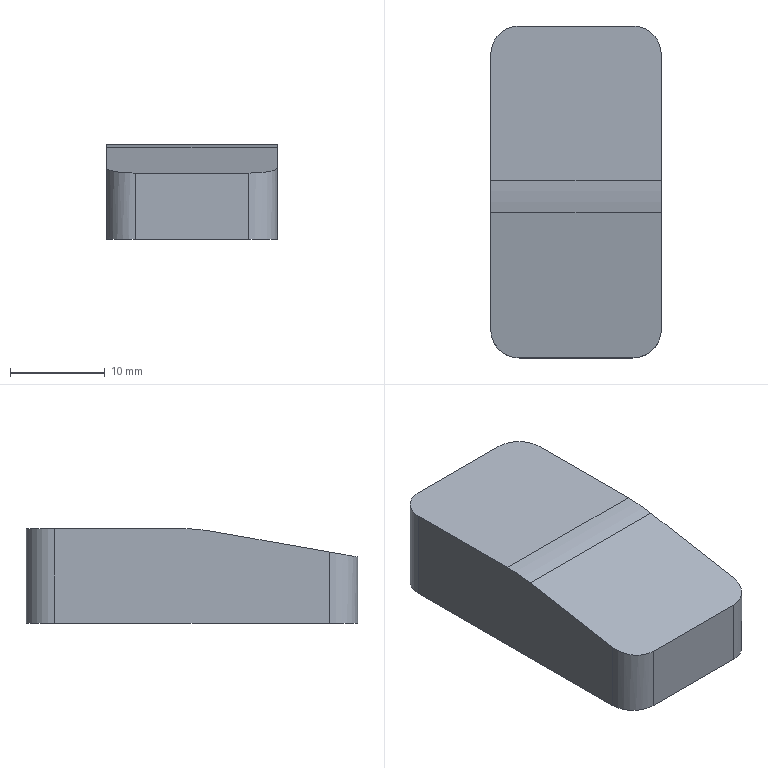Part | STEP file | Tube necking machine_id402_x_t | 1 solid | 12 faces | box 18 x 35 x 10 mm | volume 5773 mm3 | plane 7 | cylinder 5 | commonest cylinder face diameters 6 x4 39 x1
STEP:
#1=CARTESIAN_POINT('',(0.,0.,0.));
#2=DIRECTION('',(0.,0.,1.));
#3=DIRECTION('',(1.,0.,0.));
#4=AXIS2_PLACEMENT_3D('',#1,#2,#3);
#5=CARTESIAN_POINT('',(-9.,-95.,180.));
#6=VERTEX_POINT('',#5);
#7=CARTESIAN_POINT('',(-9.,-124.,180.));
#8=VERTEX_POINT('',#7);
#9=CARTESIAN_POINT('',(-9.,-92.,180.));
#10=DIRECTION('',(0.,-1.,0.));
#11=VECTOR('',#10,1.);
#12=LINE('',#9,#11);
#13=CARTESIAN_POINT('',(-9.,-92.,190.));
#14=DIRECTION('',(1.,0.,0.));
#15=DIRECTION('',(0.,0.,-1.));
#16=AXIS2_PLACEMENT_3D('',#13,#14,#15);
#17=PLANE('',#16);
#18=CARTESIAN_POINT('',(10.,0.));
#19=DIRECTION('',(0.,-1.));
#20=VECTOR('',#19,1.);
#21=LINE('',#18,#20);
#22=(GEOMETRIC_REPRESENTATION_CONTEXT(2)PARAMETRIC_REPRESENTATION_CONTEXT()REPRESENTATION_CONTEXT('',''));
#23=DEFINITIONAL_REPRESENTATION('',(#21),#22);
#24=PCURVE('',#17,#23);
#25=CARTESIAN_POINT('',(0.,0.,180.));
#26=DIRECTION('',(0.,0.,1.));
#27=DIRECTION('',(1.,0.,0.));
#28=AXIS2_PLACEMENT_3D('',#25,#26,#27);
#29=PLANE('',#28);
#30=CARTESIAN_POINT('',(-9.,-92.));
#31=DIRECTION('',(0.,-1.));
#32=VECTOR('',#31,1.);
#33=LINE('',#30,#32);
#34=(GEOMETRIC_REPRESENTATION_CONTEXT(2)PARAMETRIC_REPRESENTATION_CONTEXT()REPRESENTATION_CONTEXT('',''));
#35=DEFINITIONAL_REPRESENTATION('',(#33),#34);
#36=PCURVE('',#29,#35);
#37=SURFACE_CURVE('',#12,(#24,#36),.PCURVE_S1.);
#38=EDGE_CURVE('',#6,#8,#37,.T.);
#39=ORIENTED_EDGE('',*,*,#38,.T.);
#40=CARTESIAN_POINT('',(-9.,-124.,187.529));
#41=VERTEX_POINT('',#40);
#42=CARTESIAN_POINT('',(-9.,-124.,190.));
#43=DIRECTION('',(0.,0.,1.));
#44=VECTOR('',#43,1.);
#45=LINE('',#42,#44);
#46=CARTESIAN_POINT('',(0.,-32.));
#47=DIRECTION('',(-1.,0.));
#48=VECTOR('',#47,1.);
#49=LINE('',#46,#48);
#50=(GEOMETRIC_REPRESENTATION_CONTEXT(2)PARAMETRIC_REPRESENTATION_CONTEXT()REPRESENTATION_CONTEXT('',''));
#51=DEFINITIONAL_REPRESENTATION('',(#49),#50);
#52=PCURVE('',#17,#51);
#53=CARTESIAN_POINT('',(-6.,-124.,190.));
#54=DIRECTION('',(0.,0.,-1.));
#55=DIRECTION('',(-1.,0.,0.));
#56=AXIS2_PLACEMENT_3D('',#53,#54,#55);
#57=CYLINDRICAL_SURFACE('',#56,3.);
#58=CARTESIAN_POINT('',(6.283,0.));
#59=DIRECTION('',(0.,-1.));
#60=VECTOR('',#59,1.);
#61=LINE('',#58,#60);
#62=(GEOMETRIC_REPRESENTATION_CONTEXT(2)PARAMETRIC_REPRESENTATION_CONTEXT()REPRESENTATION_CONTEXT('',''));
#63=DEFINITIONAL_REPRESENTATION('',(#61),#62);
#64=PCURVE('',#57,#63);
#65=SURFACE_CURVE('',#45,(#52,#64),.PCURVE_S1.);
#66=EDGE_CURVE('',#8,#41,#65,.T.);
#67=ORIENTED_EDGE('',*,*,#66,.T.);
#68=CARTESIAN_POINT('',(-9.,-111.681,189.703));
#69=VERTEX_POINT('',#68);
#70=CARTESIAN_POINT('',(-9.,-110.,190.));
#71=DIRECTION('',(0.,0.9848,0.1738));
#72=VECTOR('',#71,1.);
#73=LINE('',#70,#72);
#74=CARTESIAN_POINT('',(0.,-18.));
#75=DIRECTION('',(-0.1738,0.9848));
#76=VECTOR('',#75,1.);
#77=LINE('',#74,#76);
#78=(GEOMETRIC_REPRESENTATION_CONTEXT(2)PARAMETRIC_REPRESENTATION_CONTEXT()REPRESENTATION_CONTEXT('',''));
#79=DEFINITIONAL_REPRESENTATION('',(#77),#78);
#80=PCURVE('',#17,#79);
#81=CARTESIAN_POINT('',(0.,-110.,190.));
#82=DIRECTION('',(0.,-0.1738,0.9848));
#83=DIRECTION('',(-1.,0.,0.));
#84=AXIS2_PLACEMENT_3D('',#81,#82,#83);
#85=PLANE('',#84);
#86=CARTESIAN_POINT('',(9.,0.));
#87=DIRECTION('',(0.,-1.));
#88=VECTOR('',#87,1.);
#89=LINE('',#86,#88);
#90=(GEOMETRIC_REPRESENTATION_CONTEXT(2)PARAMETRIC_REPRESENTATION_CONTEXT()REPRESENTATION_CONTEXT('',''));
#91=DEFINITIONAL_REPRESENTATION('',(#89),#90);
#92=PCURVE('',#85,#91);
#93=SURFACE_CURVE('',#73,(#80,#92),.PCURVE_S1.);
#94=EDGE_CURVE('',#41,#69,#93,.T.);
#95=ORIENTED_EDGE('',*,*,#94,.T.);
#96=CARTESIAN_POINT('',(-9.,-108.293,190.));
#97=VERTEX_POINT('',#96);
#98=CARTESIAN_POINT('',(-9.,-108.293,170.5));
#99=DIRECTION('',(-1.,0.,0.));
#100=DIRECTION('',(0.,0.,-1.));
#101=AXIS2_PLACEMENT_3D('',#98,#99,#100);
#102=CIRCLE('',#101,19.5);
#103=CARTESIAN_POINT('',(39.,-16.293));
#104=CARTESIAN_POINT('',(39.,-50.068));
#105=CARTESIAN_POINT('',(9.75,-33.18));
#106=CARTESIAN_POINT('',(-19.5,-16.293));
#107=CARTESIAN_POINT('',(9.75,0.5949));
#108=CARTESIAN_POINT('',(39.,17.482));
#109=CARTESIAN_POINT('',(39.,-16.293));
#110=(BOUNDED_CURVE()B_SPLINE_CURVE(2,(#103,#104,#105,#106,#107,#108,#109),.UNSPECIFIED.,.T.,.F.)B_SPLINE_CURVE_WITH_KNOTS((1,2,2,2,2,1),(-2.094,0.,2.094,4.189,6.283,8.378),.UNSPECIFIED.)CURVE()GEOMETRIC_REPRESENTATION_ITEM()RATIONAL_B_SPLINE_CURVE((1.,0.5,1.,0.5,1.,0.5,1.))REPRESENTATION_ITEM(''));
#111=(GEOMETRIC_REPRESENTATION_CONTEXT(2)PARAMETRIC_REPRESENTATION_CONTEXT()REPRESENTATION_CONTEXT('',''));
#112=DEFINITIONAL_REPRESENTATION('',(#110),#111);
#113=PCURVE('',#17,#112);
#114=CARTESIAN_POINT('',(0.,-108.293,170.5));
#115=DIRECTION('',(1.,0.,0.));
#116=DIRECTION('',(0.,0.,-1.));
#117=AXIS2_PLACEMENT_3D('',#114,#115,#116);
#118=CYLINDRICAL_SURFACE('',#117,19.5);
#119=CARTESIAN_POINT('',(6.283,-9.));
#120=DIRECTION('',(-1.,0.));
#121=VECTOR('',#120,1.);
#122=LINE('',#119,#121);
#123=(GEOMETRIC_REPRESENTATION_CONTEXT(2)PARAMETRIC_REPRESENTATION_CONTEXT()REPRESENTATION_CONTEXT('',''));
#124=DEFINITIONAL_REPRESENTATION('',(#122),#123);
#125=PCURVE('',#118,#124);
#126=SURFACE_CURVE('',#102,(#113,#125),.PCURVE_S1.);
#127=EDGE_CURVE('',#69,#97,#126,.T.);
#128=ORIENTED_EDGE('',*,*,#127,.T.);
#129=CARTESIAN_POINT('',(-9.,-95.,190.));
#130=VERTEX_POINT('',#129);
#131=CARTESIAN_POINT('',(-9.,-92.,190.));
#132=DIRECTION('',(0.,-1.,0.));
#133=VECTOR('',#132,1.);
#134=LINE('',#131,#133);
#135=CARTESIAN_POINT('',(0.,0.));
#136=DIRECTION('',(0.,-1.));
#137=VECTOR('',#136,1.);
#138=LINE('',#135,#137);
#139=(GEOMETRIC_REPRESENTATION_CONTEXT(2)PARAMETRIC_REPRESENTATION_CONTEXT()REPRESENTATION_CONTEXT('',''));
#140=DEFINITIONAL_REPRESENTATION('',(#138),#139);
#141=PCURVE('',#17,#140);
#142=CARTESIAN_POINT('',(0.,0.,190.));
#143=DIRECTION('',(0.,0.,1.));
#144=DIRECTION('',(1.,0.,0.));
#145=AXIS2_PLACEMENT_3D('',#142,#143,#144);
#146=PLANE('',#145);
#147=CARTESIAN_POINT('',(-9.,-92.));
#148=DIRECTION('',(0.,-1.));
#149=VECTOR('',#148,1.);
#150=LINE('',#147,#149);
#151=(GEOMETRIC_REPRESENTATION_CONTEXT(2)PARAMETRIC_REPRESENTATION_CONTEXT()REPRESENTATION_CONTEXT('',''));
#152=DEFINITIONAL_REPRESENTATION('',(#150),#151);
#153=PCURVE('',#146,#152);
#154=SURFACE_CURVE('',#134,(#141,#153),.PCURVE_S1.);
#155=EDGE_CURVE('',#130,#97,#154,.T.);
#156=ORIENTED_EDGE('',*,*,#155,.F.);
#157=CARTESIAN_POINT('',(-9.,-95.,190.));
#158=DIRECTION('',(0.,0.,-1.));
#159=VECTOR('',#158,1.);
#160=LINE('',#157,#159);
#161=CARTESIAN_POINT('',(0.,-3.));
#162=DIRECTION('',(1.,0.));
#163=VECTOR('',#162,1.);
#164=LINE('',#161,#163);
#165=(GEOMETRIC_REPRESENTATION_CONTEXT(2)PARAMETRIC_REPRESENTATION_CONTEXT()REPRESENTATION_CONTEXT('',''));
#166=DEFINITIONAL_REPRESENTATION('',(#164),#165);
#167=PCURVE('',#17,#166);
#168=CARTESIAN_POINT('',(-6.,-95.,190.));
#169=DIRECTION('',(0.,0.,-1.));
#170=DIRECTION('',(-1.,0.,0.));
#171=AXIS2_PLACEMENT_3D('',#168,#169,#170);
#172=CYLINDRICAL_SURFACE('',#171,3.);
#173=CARTESIAN_POINT('',(0.,0.));
#174=DIRECTION('',(0.,1.));
#175=VECTOR('',#174,1.);
#176=LINE('',#173,#175);
#177=(GEOMETRIC_REPRESENTATION_CONTEXT(2)PARAMETRIC_REPRESENTATION_CONTEXT()REPRESENTATION_CONTEXT('',''));
#178=DEFINITIONAL_REPRESENTATION('',(#176),#177);
#179=PCURVE('',#172,#178);
#180=SURFACE_CURVE('',#160,(#167,#179),.PCURVE_S1.);
#181=EDGE_CURVE('',#130,#6,#180,.T.);
#182=ORIENTED_EDGE('',*,*,#181,.T.);
#183=EDGE_LOOP('',(#39,#67,#95,#128,#156,#182));
#184=FACE_BOUND('',#183,.T.);
#185=ADVANCED_FACE('',(#184),#17,.F.);
#186=CARTESIAN_POINT('',(-6.,-127.,180.));
#187=VERTEX_POINT('',#186);
#188=CARTESIAN_POINT('',(6.,-127.,180.));
#189=VERTEX_POINT('',#188);
#190=CARTESIAN_POINT('',(-9.,-127.,180.));
#191=DIRECTION('',(1.,0.,0.));
#192=VECTOR('',#191,1.);
#193=LINE('',#190,#192);
#194=CARTESIAN_POINT('',(-9.,-127.,190.));
#195=DIRECTION('',(0.,1.,0.));
#196=DIRECTION('',(0.,0.,1.));
#197=AXIS2_PLACEMENT_3D('',#194,#195,#196);
#198=PLANE('',#197);
#199=CARTESIAN_POINT('',(-10.,0.));
#200=DIRECTION('',(0.,1.));
#201=VECTOR('',#200,1.);
#202=LINE('',#199,#201);
#203=(GEOMETRIC_REPRESENTATION_CONTEXT(2)PARAMETRIC_REPRESENTATION_CONTEXT()REPRESENTATION_CONTEXT('',''));
#204=DEFINITIONAL_REPRESENTATION('',(#202),#203);
#205=PCURVE('',#198,#204);
#206=CARTESIAN_POINT('',(-9.,-127.));
#207=DIRECTION('',(1.,0.));
#208=VECTOR('',#207,1.);
#209=LINE('',#206,#208);
#210=(GEOMETRIC_REPRESENTATION_CONTEXT(2)PARAMETRIC_REPRESENTATION_CONTEXT()REPRESENTATION_CONTEXT('',''));
#211=DEFINITIONAL_REPRESENTATION('',(#209),#210);
#212=PCURVE('',#29,#211);
#213=SURFACE_CURVE('',#193,(#205,#212),.PCURVE_S1.);
#214=EDGE_CURVE('',#187,#189,#213,.T.);
#215=ORIENTED_EDGE('',*,*,#214,.T.);
#216=CARTESIAN_POINT('',(6.,-127.,187.));
#217=VERTEX_POINT('',#216);
#218=CARTESIAN_POINT('',(6.,-127.,190.));
#219=DIRECTION('',(0.,0.,1.));
#220=VECTOR('',#219,1.);
#221=LINE('',#218,#220);
#222=CARTESIAN_POINT('',(0.,15.));
#223=DIRECTION('',(1.,0.));
#224=VECTOR('',#223,1.);
#225=LINE('',#222,#224);
#226=(GEOMETRIC_REPRESENTATION_CONTEXT(2)PARAMETRIC_REPRESENTATION_CONTEXT()REPRESENTATION_CONTEXT('',''));
#227=DEFINITIONAL_REPRESENTATION('',(#225),#226);
#228=PCURVE('',#198,#227);
#229=CARTESIAN_POINT('',(6.,-124.,190.));
#230=DIRECTION('',(0.,0.,-1.));
#231=DIRECTION('',(-1.,0.,0.));
#232=AXIS2_PLACEMENT_3D('',#229,#230,#231);
#233=CYLINDRICAL_SURFACE('',#232,3.);
#234=CARTESIAN_POINT('',(4.712,0.));
#235=DIRECTION('',(0.,-1.));
#236=VECTOR('',#235,1.);
#237=LINE('',#234,#236);
#238=(GEOMETRIC_REPRESENTATION_CONTEXT(2)PARAMETRIC_REPRESENTATION_CONTEXT()REPRESENTATION_CONTEXT('',''));
#239=DEFINITIONAL_REPRESENTATION('',(#237),#238);
#240=PCURVE('',#233,#239);
#241=SURFACE_CURVE('',#221,(#228,#240),.PCURVE_S1.);
#242=EDGE_CURVE('',#189,#217,#241,.T.);
#243=ORIENTED_EDGE('',*,*,#242,.T.);
#244=CARTESIAN_POINT('',(-6.,-127.,187.));
#245=VERTEX_POINT('',#244);
#246=CARTESIAN_POINT('',(-9.,-127.,187.));
#247=DIRECTION('',(-1.,0.,0.));
#248=VECTOR('',#247,1.);
#249=LINE('',#246,#248);
#250=CARTESIAN_POINT('',(-3.,0.));
#251=DIRECTION('',(0.,-1.));
#252=VECTOR('',#251,1.);
#253=LINE('',#250,#252);
#254=(GEOMETRIC_REPRESENTATION_CONTEXT(2)PARAMETRIC_REPRESENTATION_CONTEXT()REPRESENTATION_CONTEXT('',''));
#255=DEFINITIONAL_REPRESENTATION('',(#253),#254);
#256=PCURVE('',#198,#255);
#257=CARTESIAN_POINT('',(9.,17.263));
#258=DIRECTION('',(1.,0.));
#259=VECTOR('',#258,1.);
#260=LINE('',#257,#259);
#261=(GEOMETRIC_REPRESENTATION_CONTEXT(2)PARAMETRIC_REPRESENTATION_CONTEXT()REPRESENTATION_CONTEXT('',''));
#262=DEFINITIONAL_REPRESENTATION('',(#260),#261);
#263=PCURVE('',#85,#262);
#264=SURFACE_CURVE('',#249,(#256,#263),.PCURVE_S1.);
#265=EDGE_CURVE('',#217,#245,#264,.T.);
#266=ORIENTED_EDGE('',*,*,#265,.T.);
#267=CARTESIAN_POINT('',(-6.,-127.,190.));
#268=DIRECTION('',(0.,0.,-1.));
#269=VECTOR('',#268,1.);
#270=LINE('',#267,#269);
#271=CARTESIAN_POINT('',(0.,3.));
#272=DIRECTION('',(-1.,0.));
#273=VECTOR('',#272,1.);
#274=LINE('',#271,#273);
#275=(GEOMETRIC_REPRESENTATION_CONTEXT(2)PARAMETRIC_REPRESENTATION_CONTEXT()REPRESENTATION_CONTEXT('',''));
#276=DEFINITIONAL_REPRESENTATION('',(#274),#275);
#277=PCURVE('',#198,#276);
#278=CARTESIAN_POINT('',(4.712,0.));
#279=DIRECTION('',(0.,1.));
#280=VECTOR('',#279,1.);
#281=LINE('',#278,#280);
#282=(GEOMETRIC_REPRESENTATION_CONTEXT(2)PARAMETRIC_REPRESENTATION_CONTEXT()REPRESENTATION_CONTEXT('',''));
#283=DEFINITIONAL_REPRESENTATION('',(#281),#282);
#284=PCURVE('',#57,#283);
#285=SURFACE_CURVE('',#270,(#277,#284),.PCURVE_S1.);
#286=EDGE_CURVE('',#245,#187,#285,.T.);
#287=ORIENTED_EDGE('',*,*,#286,.T.);
#288=EDGE_LOOP('',(#215,#243,#266,#287));
#289=FACE_BOUND('',#288,.T.);
#290=ADVANCED_FACE('',(#289),#198,.F.);
#291=CARTESIAN_POINT('',(9.,-111.681,189.703));
#292=VERTEX_POINT('',#291);
#293=CARTESIAN_POINT('',(9.,-124.,187.529));
#294=VERTEX_POINT('',#293);
#295=CARTESIAN_POINT('',(9.,-110.,190.));
#296=DIRECTION('',(0.,-0.9848,-0.1738));
#297=VECTOR('',#296,1.);
#298=LINE('',#295,#297);
#299=CARTESIAN_POINT('',(9.,-127.,190.));
#300=DIRECTION('',(-1.,0.,0.));
#301=DIRECTION('',(0.,0.,1.));
#302=AXIS2_PLACEMENT_3D('',#299,#300,#301);
#303=PLANE('',#302);
#304=CARTESIAN_POINT('',(0.,17.));
#305=DIRECTION('',(-0.1738,-0.9848));
#306=VECTOR('',#305,1.);
#307=LINE('',#304,#306);
#308=(GEOMETRIC_REPRESENTATION_CONTEXT(2)PARAMETRIC_REPRESENTATION_CONTEXT()REPRESENTATION_CONTEXT('',''));
#309=DEFINITIONAL_REPRESENTATION('',(#307),#308);
#310=PCURVE('',#303,#309);
#311=CARTESIAN_POINT('',(-9.,0.));
#312=DIRECTION('',(0.,1.));
#313=VECTOR('',#312,1.);
#314=LINE('',#311,#313);
#315=(GEOMETRIC_REPRESENTATION_CONTEXT(2)PARAMETRIC_REPRESENTATION_CONTEXT()REPRESENTATION_CONTEXT('',''));
#316=DEFINITIONAL_REPRESENTATION('',(#314),#315);
#317=PCURVE('',#85,#316);
#318=SURFACE_CURVE('',#298,(#310,#317),.PCURVE_S1.);
#319=EDGE_CURVE('',#292,#294,#318,.T.);
#320=ORIENTED_EDGE('',*,*,#319,.T.);
#321=CARTESIAN_POINT('',(9.,-124.,180.));
#322=VERTEX_POINT('',#321);
#323=CARTESIAN_POINT('',(9.,-124.,190.));
#324=DIRECTION('',(0.,0.,-1.));
#325=VECTOR('',#324,1.);
#326=LINE('',#323,#325);
#327=CARTESIAN_POINT('',(0.,3.));
#328=DIRECTION('',(-1.,0.));
#329=VECTOR('',#328,1.);
#330=LINE('',#327,#329);
#331=(GEOMETRIC_REPRESENTATION_CONTEXT(2)PARAMETRIC_REPRESENTATION_CONTEXT()REPRESENTATION_CONTEXT('',''));
#332=DEFINITIONAL_REPRESENTATION('',(#330),#331);
#333=PCURVE('',#303,#332);
#334=CARTESIAN_POINT('',(3.142,0.));
#335=DIRECTION('',(0.,1.));
#336=VECTOR('',#335,1.);
#337=LINE('',#334,#336);
#338=(GEOMETRIC_REPRESENTATION_CONTEXT(2)PARAMETRIC_REPRESENTATION_CONTEXT()REPRESENTATION_CONTEXT('',''));
#339=DEFINITIONAL_REPRESENTATION('',(#337),#338);
#340=PCURVE('',#233,#339);
#341=SURFACE_CURVE('',#326,(#333,#340),.PCURVE_S1.);
#342=EDGE_CURVE('',#294,#322,#341,.T.);
#343=ORIENTED_EDGE('',*,*,#342,.T.);
#344=CARTESIAN_POINT('',(9.,-95.,180.));
#345=VERTEX_POINT('',#344);
#346=CARTESIAN_POINT('',(9.,-127.,180.));
#347=DIRECTION('',(0.,1.,0.));
#348=VECTOR('',#347,1.);
#349=LINE('',#346,#348);
#350=CARTESIAN_POINT('',(-10.,0.));
#351=DIRECTION('',(0.,1.));
#352=VECTOR('',#351,1.);
#353=LINE('',#350,#352);
#354=(GEOMETRIC_REPRESENTATION_CONTEXT(2)PARAMETRIC_REPRESENTATION_CONTEXT()REPRESENTATION_CONTEXT('',''));
#355=DEFINITIONAL_REPRESENTATION('',(#353),#354);
#356=PCURVE('',#303,#355);
#357=CARTESIAN_POINT('',(9.,-127.));
#358=DIRECTION('',(0.,1.));
#359=VECTOR('',#358,1.);
#360=LINE('',#357,#359);
#361=(GEOMETRIC_REPRESENTATION_CONTEXT(2)PARAMETRIC_REPRESENTATION_CONTEXT()REPRESENTATION_CONTEXT('',''));
#362=DEFINITIONAL_REPRESENTATION('',(#360),#361);
#363=PCURVE('',#29,#362);
#364=SURFACE_CURVE('',#349,(#356,#363),.PCURVE_S1.);
#365=EDGE_CURVE('',#322,#345,#364,.T.);
#366=ORIENTED_EDGE('',*,*,#365,.T.);
#367=CARTESIAN_POINT('',(9.,-95.,190.));
#368=VERTEX_POINT('',#367);
#369=CARTESIAN_POINT('',(9.,-95.,190.));
#370=DIRECTION('',(0.,0.,1.));
#371=VECTOR('',#370,1.);
#372=LINE('',#369,#371);
#373=CARTESIAN_POINT('',(0.,32.));
#374=DIRECTION('',(1.,0.));
#375=VECTOR('',#374,1.);
#376=LINE('',#373,#375);
#377=(GEOMETRIC_REPRESENTATION_CONTEXT(2)PARAMETRIC_REPRESENTATION_CONTEXT()REPRESENTATION_CONTEXT('',''));
#378=DEFINITIONAL_REPRESENTATION('',(#376),#377);
#379=PCURVE('',#303,#378);
#380=CARTESIAN_POINT('',(6.,-95.,190.));
#381=DIRECTION('',(0.,0.,-1.));
#382=DIRECTION('',(-1.,0.,0.));
#383=AXIS2_PLACEMENT_3D('',#380,#381,#382);
#384=CYLINDRICAL_SURFACE('',#383,3.);
#385=CARTESIAN_POINT('',(3.142,0.));
#386=DIRECTION('',(0.,-1.));
#387=VECTOR('',#386,1.);
#388=LINE('',#385,#387);
#389=(GEOMETRIC_REPRESENTATION_CONTEXT(2)PARAMETRIC_REPRESENTATION_CONTEXT()REPRESENTATION_CONTEXT('',''));
#390=DEFINITIONAL_REPRESENTATION('',(#388),#389);
#391=PCURVE('',#384,#390);
#392=SURFACE_CURVE('',#372,(#379,#391),.PCURVE_S1.);
#393=EDGE_CURVE('',#345,#368,#392,.T.);
#394=ORIENTED_EDGE('',*,*,#393,.T.);
#395=CARTESIAN_POINT('',(9.,-108.293,190.));
#396=VERTEX_POINT('',#395);
#397=CARTESIAN_POINT('',(9.,-127.,190.));
#398=DIRECTION('',(0.,1.,0.));
#399=VECTOR('',#398,1.);
#400=LINE('',#397,#399);
#401=CARTESIAN_POINT('',(0.,0.));
#402=DIRECTION('',(0.,1.));
#403=VECTOR('',#402,1.);
#404=LINE('',#401,#403);
#405=(GEOMETRIC_REPRESENTATION_CONTEXT(2)PARAMETRIC_REPRESENTATION_CONTEXT()REPRESENTATION_CONTEXT('',''));
#406=DEFINITIONAL_REPRESENTATION('',(#404),#405);
#407=PCURVE('',#303,#406);
#408=CARTESIAN_POINT('',(9.,-127.));
#409=DIRECTION('',(0.,1.));
#410=VECTOR('',#409,1.);
#411=LINE('',#408,#410);
#412=(GEOMETRIC_REPRESENTATION_CONTEXT(2)PARAMETRIC_REPRESENTATION_CONTEXT()REPRESENTATION_CONTEXT('',''));
#413=DEFINITIONAL_REPRESENTATION('',(#411),#412);
#414=PCURVE('',#146,#413);
#415=SURFACE_CURVE('',#400,(#407,#414),.PCURVE_S1.);
#416=EDGE_CURVE('',#396,#368,#415,.T.);
#417=ORIENTED_EDGE('',*,*,#416,.F.);
#418=CARTESIAN_POINT('',(9.,-108.293,170.5));
#419=DIRECTION('',(1.,0.,0.));
#420=DIRECTION('',(0.,0.,1.));
#421=AXIS2_PLACEMENT_3D('',#418,#419,#420);
#422=CIRCLE('',#421,19.5);
#423=CARTESIAN_POINT('',(0.,18.707));
#424=CARTESIAN_POINT('',(0.,-15.068));
#425=CARTESIAN_POINT('',(-29.25,1.82));
#426=CARTESIAN_POINT('',(-58.5,18.707));
#427=CARTESIAN_POINT('',(-29.25,35.595));
#428=CARTESIAN_POINT('',(0.,52.482));
#429=CARTESIAN_POINT('',(0.,18.707));
#430=(BOUNDED_CURVE()B_SPLINE_CURVE(2,(#423,#424,#425,#426,#427,#428,#429),.UNSPECIFIED.,.T.,.F.)B_SPLINE_CURVE_WITH_KNOTS((1,2,2,2,2,1),(-2.094,0.,2.094,4.189,6.283,8.378),.UNSPECIFIED.)CURVE()GEOMETRIC_REPRESENTATION_ITEM()RATIONAL_B_SPLINE_CURVE((1.,0.5,1.,0.5,1.,0.5,1.))REPRESENTATION_ITEM(''));
#431=(GEOMETRIC_REPRESENTATION_CONTEXT(2)PARAMETRIC_REPRESENTATION_CONTEXT()REPRESENTATION_CONTEXT('',''));
#432=DEFINITIONAL_REPRESENTATION('',(#430),#431);
#433=PCURVE('',#303,#432);
#434=CARTESIAN_POINT('',(3.142,9.));
#435=DIRECTION('',(1.,0.));
#436=VECTOR('',#435,1.);
#437=LINE('',#434,#436);
#438=(GEOMETRIC_REPRESENTATION_CONTEXT(2)PARAMETRIC_REPRESENTATION_CONTEXT()REPRESENTATION_CONTEXT('',''));
#439=DEFINITIONAL_REPRESENTATION('',(#437),#438);
#440=PCURVE('',#118,#439);
#441=SURFACE_CURVE('',#422,(#433,#440),.PCURVE_S1.);
#442=EDGE_CURVE('',#396,#292,#441,.T.);
#443=ORIENTED_EDGE('',*,*,#442,.T.);
#444=EDGE_LOOP('',(#320,#343,#366,#394,#417,#443));
#445=FACE_BOUND('',#444,.T.);
#446=ADVANCED_FACE('',(#445),#303,.F.);
#447=CARTESIAN_POINT('',(6.,-92.,180.));
#448=VERTEX_POINT('',#447);
#449=CARTESIAN_POINT('',(-6.,-92.,180.));
#450=VERTEX_POINT('',#449);
#451=CARTESIAN_POINT('',(9.,-92.,180.));
#452=DIRECTION('',(-1.,0.,0.));
#453=VECTOR('',#452,1.);
#454=LINE('',#451,#453);
#455=CARTESIAN_POINT('',(9.,-92.,190.));
#456=DIRECTION('',(0.,-1.,0.));
#457=DIRECTION('',(0.,0.,-1.));
#458=AXIS2_PLACEMENT_3D('',#455,#456,#457);
#459=PLANE('',#458);
#460=CARTESIAN_POINT('',(10.,0.));
#461=DIRECTION('',(0.,-1.));
#462=VECTOR('',#461,1.);
#463=LINE('',#460,#462);
#464=(GEOMETRIC_REPRESENTATION_CONTEXT(2)PARAMETRIC_REPRESENTATION_CONTEXT()REPRESENTATION_CONTEXT('',''));
#465=DEFINITIONAL_REPRESENTATION('',(#463),#464);
#466=PCURVE('',#459,#465);
#467=CARTESIAN_POINT('',(9.,-92.));
#468=DIRECTION('',(-1.,0.));
#469=VECTOR('',#468,1.);
#470=LINE('',#467,#469);
#471=(GEOMETRIC_REPRESENTATION_CONTEXT(2)PARAMETRIC_REPRESENTATION_CONTEXT()REPRESENTATION_CONTEXT('',''));
#472=DEFINITIONAL_REPRESENTATION('',(#470),#471);
#473=PCURVE('',#29,#472);
#474=SURFACE_CURVE('',#454,(#466,#473),.PCURVE_S1.);
#475=EDGE_CURVE('',#448,#450,#474,.T.);
#476=ORIENTED_EDGE('',*,*,#475,.T.);
#477=CARTESIAN_POINT('',(-6.,-92.,190.));
#478=VERTEX_POINT('',#477);
#479=CARTESIAN_POINT('',(-6.,-92.,190.));
#480=DIRECTION('',(0.,0.,1.));
#481=VECTOR('',#480,1.);
#482=LINE('',#479,#481);
#483=CARTESIAN_POINT('',(0.,-15.));
#484=DIRECTION('',(-1.,0.));
#485=VECTOR('',#484,1.);
#486=LINE('',#483,#485);
#487=(GEOMETRIC_REPRESENTATION_CONTEXT(2)PARAMETRIC_REPRESENTATION_CONTEXT()REPRESENTATION_CONTEXT('',''));
#488=DEFINITIONAL_REPRESENTATION('',(#486),#487);
#489=PCURVE('',#459,#488);
#490=CARTESIAN_POINT('',(1.571,0.));
#491=DIRECTION('',(0.,-1.));
#492=VECTOR('',#491,1.);
#493=LINE('',#490,#492);
#494=(GEOMETRIC_REPRESENTATION_CONTEXT(2)PARAMETRIC_REPRESENTATION_CONTEXT()REPRESENTATION_CONTEXT('',''));
#495=DEFINITIONAL_REPRESENTATION('',(#493),#494);
#496=PCURVE('',#172,#495);
#497=SURFACE_CURVE('',#482,(#489,#496),.PCURVE_S1.);
#498=EDGE_CURVE('',#450,#478,#497,.T.);
#499=ORIENTED_EDGE('',*,*,#498,.T.);
#500=CARTESIAN_POINT('',(6.,-92.,190.));
#501=VERTEX_POINT('',#500);
#502=CARTESIAN_POINT('',(9.,-92.,190.));
#503=DIRECTION('',(-1.,0.,0.));
#504=VECTOR('',#503,1.);
#505=LINE('',#502,#504);
#506=CARTESIAN_POINT('',(0.,0.));
#507=DIRECTION('',(0.,-1.));
#508=VECTOR('',#507,1.);
#509=LINE('',#506,#508);
#510=(GEOMETRIC_REPRESENTATION_CONTEXT(2)PARAMETRIC_REPRESENTATION_CONTEXT()REPRESENTATION_CONTEXT('',''));
#511=DEFINITIONAL_REPRESENTATION('',(#509),#510);
#512=PCURVE('',#459,#511);
#513=CARTESIAN_POINT('',(9.,-92.));
#514=DIRECTION('',(-1.,0.));
#515=VECTOR('',#514,1.);
#516=LINE('',#513,#515);
#517=(GEOMETRIC_REPRESENTATION_CONTEXT(2)PARAMETRIC_REPRESENTATION_CONTEXT()REPRESENTATION_CONTEXT('',''));
#518=DEFINITIONAL_REPRESENTATION('',(#516),#517);
#519=PCURVE('',#146,#518);
#520=SURFACE_CURVE('',#505,(#512,#519),.PCURVE_S1.);
#521=EDGE_CURVE('',#501,#478,#520,.T.);
#522=ORIENTED_EDGE('',*,*,#521,.F.);
#523=CARTESIAN_POINT('',(6.,-92.,190.));
#524=DIRECTION('',(0.,0.,-1.));
#525=VECTOR('',#524,1.);
#526=LINE('',#523,#525);
#527=CARTESIAN_POINT('',(0.,-3.));
#528=DIRECTION('',(1.,0.));
#529=VECTOR('',#528,1.);
#530=LINE('',#527,#529);
#531=(GEOMETRIC_REPRESENTATION_CONTEXT(2)PARAMETRIC_REPRESENTATION_CONTEXT()REPRESENTATION_CONTEXT('',''));
#532=DEFINITIONAL_REPRESENTATION('',(#530),#531);
#533=PCURVE('',#459,#532);
#534=CARTESIAN_POINT('',(1.571,0.));
#535=DIRECTION('',(0.,1.));
#536=VECTOR('',#535,1.);
#537=LINE('',#534,#536);
#538=(GEOMETRIC_REPRESENTATION_CONTEXT(2)PARAMETRIC_REPRESENTATION_CONTEXT()REPRESENTATION_CONTEXT('',''));
#539=DEFINITIONAL_REPRESENTATION('',(#537),#538);
#540=PCURVE('',#384,#539);
#541=SURFACE_CURVE('',#526,(#533,#540),.PCURVE_S1.);
#542=EDGE_CURVE('',#501,#448,#541,.T.);
#543=ORIENTED_EDGE('',*,*,#542,.T.);
#544=EDGE_LOOP('',(#476,#499,#522,#543));
#545=FACE_BOUND('',#544,.T.);
#546=ADVANCED_FACE('',(#545),#459,.F.);
#547=ORIENTED_EDGE('',*,*,#155,.T.);
#548=CARTESIAN_POINT('',(0.,-108.293,190.));
#549=DIRECTION('',(1.,0.,0.));
#550=VECTOR('',#549,1.);
#551=LINE('',#548,#550);
#552=CARTESIAN_POINT('',(0.,-108.293));
#553=DIRECTION('',(1.,0.));
#554=VECTOR('',#553,1.);
#555=LINE('',#552,#554);
#556=(GEOMETRIC_REPRESENTATION_CONTEXT(2)PARAMETRIC_REPRESENTATION_CONTEXT()REPRESENTATION_CONTEXT('',''));
#557=DEFINITIONAL_REPRESENTATION('',(#555),#556);
#558=PCURVE('',#146,#557);
#559=CARTESIAN_POINT('',(3.142,0.));
#560=DIRECTION('',(0.,1.));
#561=VECTOR('',#560,1.);
#562=LINE('',#559,#561);
#563=(GEOMETRIC_REPRESENTATION_CONTEXT(2)PARAMETRIC_REPRESENTATION_CONTEXT()REPRESENTATION_CONTEXT('',''));
#564=DEFINITIONAL_REPRESENTATION('',(#562),#563);
#565=PCURVE('',#118,#564);
#566=SURFACE_CURVE('',#551,(#558,#565),.PCURVE_S1.);
#567=EDGE_CURVE('',#97,#396,#566,.T.);
#568=ORIENTED_EDGE('',*,*,#567,.T.);
#569=ORIENTED_EDGE('',*,*,#416,.T.);
#570=CARTESIAN_POINT('',(6.,-95.,190.));
#571=DIRECTION('',(0.,0.,1.));
#572=DIRECTION('',(1.,0.,0.));
#573=AXIS2_PLACEMENT_3D('',#570,#571,#572);
#574=CIRCLE('',#573,3.);
#575=CARTESIAN_POINT('',(6.,-95.));
#576=DIRECTION('',(1.,0.));
#577=AXIS2_PLACEMENT_2D('',#575,#576);
#578=CIRCLE('',#577,3.);
#579=(GEOMETRIC_REPRESENTATION_CONTEXT(2)PARAMETRIC_REPRESENTATION_CONTEXT()REPRESENTATION_CONTEXT('',''));
#580=DEFINITIONAL_REPRESENTATION('',(#578),#579);
#581=PCURVE('',#146,#580);
#582=CARTESIAN_POINT('',(3.142,0.));
#583=DIRECTION('',(-1.,0.));
#584=VECTOR('',#583,1.);
#585=LINE('',#582,#584);
#586=(GEOMETRIC_REPRESENTATION_CONTEXT(2)PARAMETRIC_REPRESENTATION_CONTEXT()REPRESENTATION_CONTEXT('',''));
#587=DEFINITIONAL_REPRESENTATION('',(#585),#586);
#588=PCURVE('',#384,#587);
#589=SURFACE_CURVE('',#574,(#581,#588),.PCURVE_S1.);
#590=EDGE_CURVE('',#368,#501,#589,.T.);
#591=ORIENTED_EDGE('',*,*,#590,.T.);
#592=ORIENTED_EDGE('',*,*,#521,.T.);
#593=CARTESIAN_POINT('',(-6.,-95.,190.));
#594=DIRECTION('',(0.,0.,1.));
#595=DIRECTION('',(1.,0.,0.));
#596=AXIS2_PLACEMENT_3D('',#593,#594,#595);
#597=CIRCLE('',#596,3.);
#598=CARTESIAN_POINT('',(-6.,-95.));
#599=DIRECTION('',(1.,0.));
#600=AXIS2_PLACEMENT_2D('',#598,#599);
#601=CIRCLE('',#600,3.);
#602=(GEOMETRIC_REPRESENTATION_CONTEXT(2)PARAMETRIC_REPRESENTATION_CONTEXT()REPRESENTATION_CONTEXT('',''));
#603=DEFINITIONAL_REPRESENTATION('',(#601),#602);
#604=PCURVE('',#146,#603);
#605=CARTESIAN_POINT('',(3.142,0.));
#606=DIRECTION('',(-1.,0.));
#607=VECTOR('',#606,1.);
#608=LINE('',#605,#607);
#609=(GEOMETRIC_REPRESENTATION_CONTEXT(2)PARAMETRIC_REPRESENTATION_CONTEXT()REPRESENTATION_CONTEXT('',''));
#610=DEFINITIONAL_REPRESENTATION('',(#608),#609);
#611=PCURVE('',#172,#610);
#612=SURFACE_CURVE('',#597,(#604,#611),.PCURVE_S1.);
#613=EDGE_CURVE('',#478,#130,#612,.T.);
#614=ORIENTED_EDGE('',*,*,#613,.T.);
#615=EDGE_LOOP('',(#547,#568,#569,#591,#592,#614));
#616=FACE_BOUND('',#615,.T.);
#617=ADVANCED_FACE('',(#616),#146,.T.);
#618=ORIENTED_EDGE('',*,*,#365,.F.);
#619=CARTESIAN_POINT('',(6.,-124.,180.));
#620=DIRECTION('',(0.,0.,-1.));
#621=DIRECTION('',(1.,0.,0.));
#622=AXIS2_PLACEMENT_3D('',#619,#620,#621);
#623=CIRCLE('',#622,3.);
#624=CARTESIAN_POINT('',(9.,-124.));
#625=CARTESIAN_POINT('',(9.,-129.196));
#626=CARTESIAN_POINT('',(4.5,-126.598));
#627=CARTESIAN_POINT('',(0.,-124.));
#628=CARTESIAN_POINT('',(4.5,-121.402));
#629=CARTESIAN_POINT('',(9.,-118.804));
#630=CARTESIAN_POINT('',(9.,-124.));
#631=(BOUNDED_CURVE()B_SPLINE_CURVE(2,(#624,#625,#626,#627,#628,#629,#630),.UNSPECIFIED.,.T.,.F.)B_SPLINE_CURVE_WITH_KNOTS((1,2,2,2,2,1),(-2.094,0.,2.094,4.189,6.283,8.378),.UNSPECIFIED.)CURVE()GEOMETRIC_REPRESENTATION_ITEM()RATIONAL_B_SPLINE_CURVE((1.,0.5,1.,0.5,1.,0.5,1.))REPRESENTATION_ITEM(''));
#632=(GEOMETRIC_REPRESENTATION_CONTEXT(2)PARAMETRIC_REPRESENTATION_CONTEXT()REPRESENTATION_CONTEXT('',''));
#633=DEFINITIONAL_REPRESENTATION('',(#631),#632);
#634=PCURVE('',#29,#633);
#635=CARTESIAN_POINT('',(3.142,10.));
#636=DIRECTION('',(1.,0.));
#637=VECTOR('',#636,1.);
#638=LINE('',#635,#637);
#639=(GEOMETRIC_REPRESENTATION_CONTEXT(2)PARAMETRIC_REPRESENTATION_CONTEXT()REPRESENTATION_CONTEXT('',''));
#640=DEFINITIONAL_REPRESENTATION('',(#638),#639);
#641=PCURVE('',#233,#640);
#642=SURFACE_CURVE('',#623,(#634,#641),.PCURVE_S1.);
#643=EDGE_CURVE('',#322,#189,#642,.T.);
#644=ORIENTED_EDGE('',*,*,#643,.T.);
#645=ORIENTED_EDGE('',*,*,#214,.F.);
#646=CARTESIAN_POINT('',(-6.,-124.,180.));
#647=DIRECTION('',(0.,0.,-1.));
#648=DIRECTION('',(1.,0.,0.));
#649=AXIS2_PLACEMENT_3D('',#646,#647,#648);
#650=CIRCLE('',#649,3.);
#651=CARTESIAN_POINT('',(-3.,-124.));
#652=CARTESIAN_POINT('',(-3.,-129.196));
#653=CARTESIAN_POINT('',(-7.5,-126.598));
#654=CARTESIAN_POINT('',(-12.,-124.));
#655=CARTESIAN_POINT('',(-7.5,-121.402));
#656=CARTESIAN_POINT('',(-3.,-118.804));
#657=CARTESIAN_POINT('',(-3.,-124.));
#658=(BOUNDED_CURVE()B_SPLINE_CURVE(2,(#651,#652,#653,#654,#655,#656,#657),.UNSPECIFIED.,.T.,.F.)B_SPLINE_CURVE_WITH_KNOTS((1,2,2,2,2,1),(-2.094,0.,2.094,4.189,6.283,8.378),.UNSPECIFIED.)CURVE()GEOMETRIC_REPRESENTATION_ITEM()RATIONAL_B_SPLINE_CURVE((1.,0.5,1.,0.5,1.,0.5,1.))REPRESENTATION_ITEM(''));
#659=(GEOMETRIC_REPRESENTATION_CONTEXT(2)PARAMETRIC_REPRESENTATION_CONTEXT()REPRESENTATION_CONTEXT('',''));
#660=DEFINITIONAL_REPRESENTATION('',(#658),#659);
#661=PCURVE('',#29,#660);
#662=CARTESIAN_POINT('',(3.142,10.));
#663=DIRECTION('',(1.,0.));
#664=VECTOR('',#663,1.);
#665=LINE('',#662,#664);
#666=(GEOMETRIC_REPRESENTATION_CONTEXT(2)PARAMETRIC_REPRESENTATION_CONTEXT()REPRESENTATION_CONTEXT('',''));
#667=DEFINITIONAL_REPRESENTATION('',(#665),#666);
#668=PCURVE('',#57,#667);
#669=SURFACE_CURVE('',#650,(#661,#668),.PCURVE_S1.);
#670=EDGE_CURVE('',#187,#8,#669,.T.);
#671=ORIENTED_EDGE('',*,*,#670,.T.);
#672=ORIENTED_EDGE('',*,*,#38,.F.);
#673=CARTESIAN_POINT('',(-6.,-95.,180.));
#674=DIRECTION('',(0.,0.,-1.));
#675=DIRECTION('',(1.,0.,0.));
#676=AXIS2_PLACEMENT_3D('',#673,#674,#675);
#677=CIRCLE('',#676,3.);
#678=CARTESIAN_POINT('',(-3.,-95.));
#679=CARTESIAN_POINT('',(-3.,-100.196));
#680=CARTESIAN_POINT('',(-7.5,-97.598));
#681=CARTESIAN_POINT('',(-12.,-95.));
#682=CARTESIAN_POINT('',(-7.5,-92.402));
#683=CARTESIAN_POINT('',(-3.,-89.804));
#684=CARTESIAN_POINT('',(-3.,-95.));
#685=(BOUNDED_CURVE()B_SPLINE_CURVE(2,(#678,#679,#680,#681,#682,#683,#684),.UNSPECIFIED.,.T.,.F.)B_SPLINE_CURVE_WITH_KNOTS((1,2,2,2,2,1),(-2.094,0.,2.094,4.189,6.283,8.378),.UNSPECIFIED.)CURVE()GEOMETRIC_REPRESENTATION_ITEM()RATIONAL_B_SPLINE_CURVE((1.,0.5,1.,0.5,1.,0.5,1.))REPRESENTATION_ITEM(''));
#686=(GEOMETRIC_REPRESENTATION_CONTEXT(2)PARAMETRIC_REPRESENTATION_CONTEXT()REPRESENTATION_CONTEXT('',''));
#687=DEFINITIONAL_REPRESENTATION('',(#685),#686);
#688=PCURVE('',#29,#687);
#689=CARTESIAN_POINT('',(-3.142,10.));
#690=DIRECTION('',(1.,0.));
#691=VECTOR('',#690,1.);
#692=LINE('',#689,#691);
#693=(GEOMETRIC_REPRESENTATION_CONTEXT(2)PARAMETRIC_REPRESENTATION_CONTEXT()REPRESENTATION_CONTEXT('',''));
#694=DEFINITIONAL_REPRESENTATION('',(#692),#693);
#695=PCURVE('',#172,#694);
#696=SURFACE_CURVE('',#677,(#688,#695),.PCURVE_S1.);
#697=EDGE_CURVE('',#6,#450,#696,.T.);
#698=ORIENTED_EDGE('',*,*,#697,.T.);
#699=ORIENTED_EDGE('',*,*,#475,.F.);
#700=CARTESIAN_POINT('',(6.,-95.,180.));
#701=DIRECTION('',(0.,0.,-1.));
#702=DIRECTION('',(1.,0.,0.));
#703=AXIS2_PLACEMENT_3D('',#700,#701,#702);
#704=CIRCLE('',#703,3.);
#705=CARTESIAN_POINT('',(9.,-95.));
#706=CARTESIAN_POINT('',(9.,-100.196));
#707=CARTESIAN_POINT('',(4.5,-97.598));
#708=CARTESIAN_POINT('',(0.,-95.));
#709=CARTESIAN_POINT('',(4.5,-92.402));
#710=CARTESIAN_POINT('',(9.,-89.804));
#711=CARTESIAN_POINT('',(9.,-95.));
#712=(BOUNDED_CURVE()B_SPLINE_CURVE(2,(#705,#706,#707,#708,#709,#710,#711),.UNSPECIFIED.,.T.,.F.)B_SPLINE_CURVE_WITH_KNOTS((1,2,2,2,2,1),(-2.094,0.,2.094,4.189,6.283,8.378),.UNSPECIFIED.)CURVE()GEOMETRIC_REPRESENTATION_ITEM()RATIONAL_B_SPLINE_CURVE((1.,0.5,1.,0.5,1.,0.5,1.))REPRESENTATION_ITEM(''));
#713=(GEOMETRIC_REPRESENTATION_CONTEXT(2)PARAMETRIC_REPRESENTATION_CONTEXT()REPRESENTATION_CONTEXT('',''));
#714=DEFINITIONAL_REPRESENTATION('',(#712),#713);
#715=PCURVE('',#29,#714);
#716=CARTESIAN_POINT('',(-3.142,10.));
#717=DIRECTION('',(1.,0.));
#718=VECTOR('',#717,1.);
#719=LINE('',#716,#718);
#720=(GEOMETRIC_REPRESENTATION_CONTEXT(2)PARAMETRIC_REPRESENTATION_CONTEXT()REPRESENTATION_CONTEXT('',''));
#721=DEFINITIONAL_REPRESENTATION('',(#719),#720);
#722=PCURVE('',#384,#721);
#723=SURFACE_CURVE('',#704,(#715,#722),.PCURVE_S1.);
#724=EDGE_CURVE('',#448,#345,#723,.T.);
#725=ORIENTED_EDGE('',*,*,#724,.T.);
#726=EDGE_LOOP('',(#618,#644,#645,#671,#672,#698,#699,#725));
#727=FACE_BOUND('',#726,.T.);
#728=ADVANCED_FACE('',(#727),#29,.F.);
#729=ORIENTED_EDGE('',*,*,#265,.F.);
#730=CARTESIAN_POINT('',(6.,-124.,187.529));
#731=DIRECTION('',(0.,-0.1738,0.9848));
#732=DIRECTION('',(0.,-0.9848,-0.1738));
#733=AXIS2_PLACEMENT_3D('',#730,#731,#732);
#734=ELLIPSE('',#733,3.046,3.);
#735=CARTESIAN_POINT('',(-6.,14.216));
#736=DIRECTION('',(0.,1.));
#737=AXIS2_PLACEMENT_2D('',#735,#736);
#738=ELLIPSE('',#737,3.046,3.);
#739=(GEOMETRIC_REPRESENTATION_CONTEXT(2)PARAMETRIC_REPRESENTATION_CONTEXT()REPRESENTATION_CONTEXT('',''));
#740=DEFINITIONAL_REPRESENTATION('',(#738),#739);
#741=PCURVE('',#85,#740);
#742=CARTESIAN_POINT('',(4.712,3.));
#743=CARTESIAN_POINT('',(4.689,3.));
#744=CARTESIAN_POINT('',(4.641,2.999));
#745=CARTESIAN_POINT('',(4.57,2.995));
#746=CARTESIAN_POINT('',(4.498,2.988));
#747=CARTESIAN_POINT('',(4.427,2.979));
#748=CARTESIAN_POINT('',(4.355,2.967));
#749=CARTESIAN_POINT('',(4.284,2.953));
#750=CARTESIAN_POINT('',(4.213,2.936));
#751=CARTESIAN_POINT('',(4.141,2.916));
#752=CARTESIAN_POINT('',(4.07,2.895));
#753=CARTESIAN_POINT('',(3.998,2.871));
#754=CARTESIAN_POINT('',(3.927,2.845));
#755=CARTESIAN_POINT('',(3.856,2.818));
#756=CARTESIAN_POINT('',(3.784,2.788));
#757=CARTESIAN_POINT('',(3.713,2.757));
#758=CARTESIAN_POINT('',(3.641,2.725));
#759=CARTESIAN_POINT('',(3.57,2.691));
#760=CARTESIAN_POINT('',(3.499,2.656));
#761=CARTESIAN_POINT('',(3.427,2.62));
#762=CARTESIAN_POINT('',(3.356,2.583));
#763=CARTESIAN_POINT('',(3.284,2.546));
#764=CARTESIAN_POINT('',(3.213,2.508));
#765=CARTESIAN_POINT('',(3.165,2.483));
#766=CARTESIAN_POINT('',(3.142,2.471));
#767=B_SPLINE_CURVE_WITH_KNOTS('',3,(#742,#743,#744,#745,#746,#747,#748,#749,#750,#751,#752,#753,#754,#755,#756,#757,#758,#759,#760,#761,#762,#763,#764,#765,#766),.UNSPECIFIED.,.F.,.F.,(4,1,1,1,1,1,1,1,1,1,1,1,1,1,1,1,1,1,1,1,1,1,4),(0.,0.0714,0.1428,0.2142,0.2856,0.357,0.4284,0.4998,0.5712,0.6426,0.714,0.7854,0.8568,0.9282,0.9996,1.071,1.142,1.214,1.285,1.357,1.428,1.499,1.571),.QUASI_UNIFORM_KNOTS.);
#768=(GEOMETRIC_REPRESENTATION_CONTEXT(2)PARAMETRIC_REPRESENTATION_CONTEXT()REPRESENTATION_CONTEXT('',''));
#769=DEFINITIONAL_REPRESENTATION('',(#767),#768);
#770=PCURVE('',#233,#769);
#771=SURFACE_CURVE('',#734,(#741,#770),.PCURVE_S1.);
#772=EDGE_CURVE('',#217,#294,#771,.T.);
#773=ORIENTED_EDGE('',*,*,#772,.T.);
#774=ORIENTED_EDGE('',*,*,#319,.F.);
#775=CARTESIAN_POINT('',(0.,-111.681,189.703));
#776=DIRECTION('',(-1.,0.,0.));
#777=VECTOR('',#776,1.);
#778=LINE('',#775,#777);
#779=CARTESIAN_POINT('',(0.,1.707));
#780=DIRECTION('',(1.,0.));
#781=VECTOR('',#780,1.);
#782=LINE('',#779,#781);
#783=(GEOMETRIC_REPRESENTATION_CONTEXT(2)PARAMETRIC_REPRESENTATION_CONTEXT()REPRESENTATION_CONTEXT('',''));
#784=DEFINITIONAL_REPRESENTATION('',(#782),#783);
#785=PCURVE('',#85,#784);
#786=CARTESIAN_POINT('',(3.316,0.));
#787=DIRECTION('',(0.,-1.));
#788=VECTOR('',#787,1.);
#789=LINE('',#786,#788);
#790=(GEOMETRIC_REPRESENTATION_CONTEXT(2)PARAMETRIC_REPRESENTATION_CONTEXT()REPRESENTATION_CONTEXT('',''));
#791=DEFINITIONAL_REPRESENTATION('',(#789),#790);
#792=PCURVE('',#118,#791);
#793=SURFACE_CURVE('',#778,(#785,#792),.PCURVE_S1.);
#794=EDGE_CURVE('',#292,#69,#793,.T.);
#795=ORIENTED_EDGE('',*,*,#794,.T.);
#796=ORIENTED_EDGE('',*,*,#94,.F.);
#797=CARTESIAN_POINT('',(-6.,-124.,187.529));
#798=DIRECTION('',(0.,-0.1738,0.9848));
#799=DIRECTION('',(0.,-0.9848,-0.1738));
#800=AXIS2_PLACEMENT_3D('',#797,#798,#799);
#801=ELLIPSE('',#800,3.046,3.);
#802=CARTESIAN_POINT('',(6.,14.216));
#803=DIRECTION('',(0.,1.));
#804=AXIS2_PLACEMENT_2D('',#802,#803);
#805=ELLIPSE('',#804,3.046,3.);
#806=(GEOMETRIC_REPRESENTATION_CONTEXT(2)PARAMETRIC_REPRESENTATION_CONTEXT()REPRESENTATION_CONTEXT('',''));
#807=DEFINITIONAL_REPRESENTATION('',(#805),#806);
#808=PCURVE('',#85,#807);
#809=CARTESIAN_POINT('',(6.283,2.471));
#810=CARTESIAN_POINT('',(6.259,2.483));
#811=CARTESIAN_POINT('',(6.212,2.508));
#812=CARTESIAN_POINT('',(6.14,2.546));
#813=CARTESIAN_POINT('',(6.069,2.583));
#814=CARTESIAN_POINT('',(5.998,2.62));
#815=CARTESIAN_POINT('',(5.926,2.656));
#816=CARTESIAN_POINT('',(5.855,2.691));
#817=CARTESIAN_POINT('',(5.783,2.725));
#818=CARTESIAN_POINT('',(5.712,2.757));
#819=CARTESIAN_POINT('',(5.641,2.788));
#820=CARTESIAN_POINT('',(5.569,2.818));
#821=CARTESIAN_POINT('',(5.498,2.845));
#822=CARTESIAN_POINT('',(5.426,2.871));
#823=CARTESIAN_POINT('',(5.355,2.895));
#824=CARTESIAN_POINT('',(5.284,2.916));
#825=CARTESIAN_POINT('',(5.212,2.936));
#826=CARTESIAN_POINT('',(5.141,2.953));
#827=CARTESIAN_POINT('',(5.069,2.967));
#828=CARTESIAN_POINT('',(4.998,2.979));
#829=CARTESIAN_POINT('',(4.927,2.988));
#830=CARTESIAN_POINT('',(4.855,2.995));
#831=CARTESIAN_POINT('',(4.784,2.999));
#832=CARTESIAN_POINT('',(4.736,3.));
#833=CARTESIAN_POINT('',(4.712,3.));
#834=B_SPLINE_CURVE_WITH_KNOTS('',3,(#809,#810,#811,#812,#813,#814,#815,#816,#817,#818,#819,#820,#821,#822,#823,#824,#825,#826,#827,#828,#829,#830,#831,#832,#833),.UNSPECIFIED.,.F.,.F.,(4,1,1,1,1,1,1,1,1,1,1,1,1,1,1,1,1,1,1,1,1,1,4),(4.712,4.784,4.855,4.927,4.998,5.069,5.141,5.212,5.284,5.355,5.426,5.498,5.569,5.641,5.712,5.783,5.855,5.926,5.998,6.069,6.14,6.212,6.283),.QUASI_UNIFORM_KNOTS.);
#835=(GEOMETRIC_REPRESENTATION_CONTEXT(2)PARAMETRIC_REPRESENTATION_CONTEXT()REPRESENTATION_CONTEXT('',''));
#836=DEFINITIONAL_REPRESENTATION('',(#834),#835);
#837=PCURVE('',#57,#836);
#838=SURFACE_CURVE('',#801,(#808,#837),.PCURVE_S1.);
#839=EDGE_CURVE('',#41,#245,#838,.T.);
#840=ORIENTED_EDGE('',*,*,#839,.T.);
#841=EDGE_LOOP('',(#729,#773,#774,#795,#796,#840));
#842=FACE_BOUND('',#841,.T.);
#843=ADVANCED_FACE('',(#842),#85,.T.);
#844=ORIENTED_EDGE('',*,*,#613,.F.);
#845=ORIENTED_EDGE('',*,*,#498,.F.);
#846=ORIENTED_EDGE('',*,*,#697,.F.);
#847=ORIENTED_EDGE('',*,*,#181,.F.);
#848=EDGE_LOOP('',(#844,#845,#846,#847));
#849=FACE_BOUND('',#848,.T.);
#850=ADVANCED_FACE('',(#849),#172,.T.);
#851=ORIENTED_EDGE('',*,*,#590,.F.);
#852=ORIENTED_EDGE('',*,*,#393,.F.);
#853=ORIENTED_EDGE('',*,*,#724,.F.);
#854=ORIENTED_EDGE('',*,*,#542,.F.);
#855=EDGE_LOOP('',(#851,#852,#853,#854));
#856=FACE_BOUND('',#855,.T.);
#857=ADVANCED_FACE('',(#856),#384,.T.);
#858=ORIENTED_EDGE('',*,*,#127,.F.);
#859=ORIENTED_EDGE('',*,*,#794,.F.);
#860=ORIENTED_EDGE('',*,*,#442,.F.);
#861=ORIENTED_EDGE('',*,*,#567,.F.);
#862=EDGE_LOOP('',(#858,#859,#860,#861));
#863=FACE_BOUND('',#862,.T.);
#864=ADVANCED_FACE('',(#863),#118,.T.);
#865=ORIENTED_EDGE('',*,*,#772,.F.);
#866=ORIENTED_EDGE('',*,*,#242,.F.);
#867=ORIENTED_EDGE('',*,*,#643,.F.);
#868=ORIENTED_EDGE('',*,*,#342,.F.);
#869=EDGE_LOOP('',(#865,#866,#867,#868));
#870=FACE_BOUND('',#869,.T.);
#871=ADVANCED_FACE('',(#870),#233,.T.);
#872=ORIENTED_EDGE('',*,*,#839,.F.);
#873=ORIENTED_EDGE('',*,*,#66,.F.);
#874=ORIENTED_EDGE('',*,*,#670,.F.);
#875=ORIENTED_EDGE('',*,*,#286,.F.);
#876=EDGE_LOOP('',(#872,#873,#874,#875));
#877=FACE_BOUND('',#876,.T.);
#878=ADVANCED_FACE('',(#877),#57,.T.);
#879=CLOSED_SHELL('',(#185,#290,#446,#546,#617,#728,#843,#850,#857,#864,#871,#878));
#880=MANIFOLD_SOLID_BREP('',#879);
#881=(LENGTH_UNIT()NAMED_UNIT(*)SI_UNIT(.MILLI.,.METRE.));
#882=UNCERTAINTY_MEASURE_WITH_UNIT(LENGTH_MEASURE(0.0000001),#881,'','');
#883=(NAMED_UNIT(*)PLANE_ANGLE_UNIT()SI_UNIT($,.RADIAN.));
#884=(NAMED_UNIT(*)SI_UNIT($,.STERADIAN.)SOLID_ANGLE_UNIT());
#885=(GEOMETRIC_REPRESENTATION_CONTEXT(3)GLOBAL_UNCERTAINTY_ASSIGNED_CONTEXT((#882))GLOBAL_UNIT_ASSIGNED_CONTEXT((#881,#883,#884))REPRESENTATION_CONTEXT('',''));
#886=ADVANCED_BREP_SHAPE_REPRESENTATION('',(#4,#880),#885);